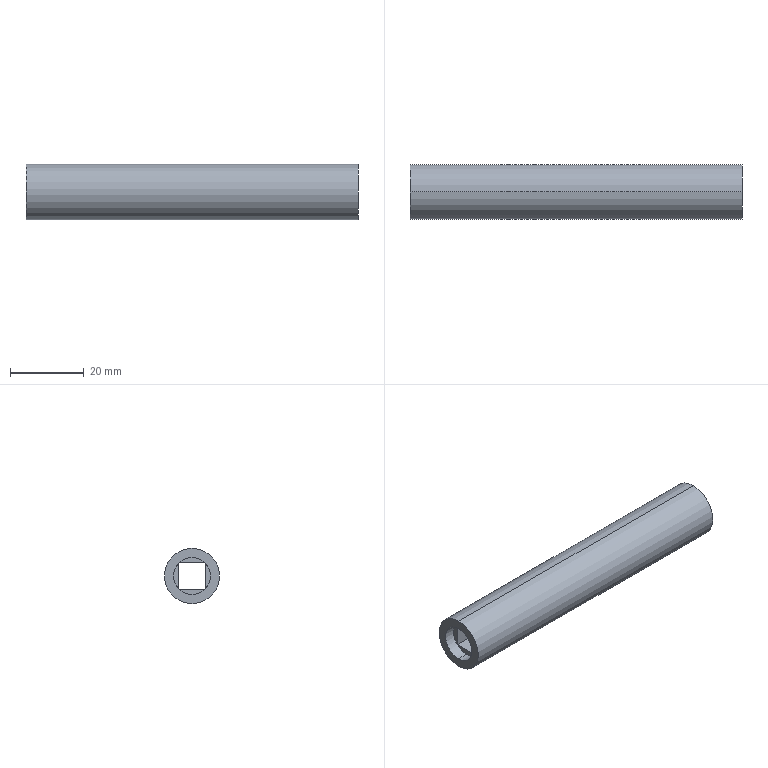Part | STEP file | Handle B | 1 solid | 18 faces | box 90 x 15 x 15 mm | volume 11283 mm3 | plane 14 | cylinder 4 | commonest cylinder face diameters 10 x2 15 x2
STEP:
#1=CARTESIAN_POINT('',(0.,0.,0.));
#2=DIRECTION('',(0.,0.,1.));
#3=DIRECTION('',(1.,0.,0.));
#4=AXIS2_PLACEMENT_3D('',#1,#2,#3);
#5=CARTESIAN_POINT('',(90.,0.,7.5));
#6=VERTEX_POINT('',#5);
#7=CARTESIAN_POINT('',(90.,0.,-7.5));
#8=VERTEX_POINT('',#7);
#9=CARTESIAN_POINT('',(90.,0.,0.));
#10=DIRECTION('',(-1.,0.,0.));
#11=DIRECTION('',(0.,0.,1.));
#12=AXIS2_PLACEMENT_3D('',#9,#10,#11);
#13=CIRCLE('',#12,7.5);
#14=CARTESIAN_POINT('',(0.,0.,0.));
#15=DIRECTION('',(-1.,0.,0.));
#16=DIRECTION('',(0.,0.,1.));
#17=AXIS2_PLACEMENT_3D('',#14,#15,#16);
#18=CYLINDRICAL_SURFACE('',#17,7.5);
#19=CARTESIAN_POINT('',(0.,-90.));
#20=DIRECTION('',(1.,0.));
#21=VECTOR('',#20,1.);
#22=LINE('',#19,#21);
#23=(GEOMETRIC_REPRESENTATION_CONTEXT(2)PARAMETRIC_REPRESENTATION_CONTEXT()REPRESENTATION_CONTEXT('',''));
#24=DEFINITIONAL_REPRESENTATION('',(#22),#23);
#25=PCURVE('',#18,#24);
#26=CARTESIAN_POINT('',(90.,7.5,0.));
#27=DIRECTION('',(-1.,0.,0.));
#28=DIRECTION('',(0.,0.,1.));
#29=AXIS2_PLACEMENT_3D('',#26,#27,#28);
#30=PLANE('',#29);
#31=CARTESIAN_POINT('',(0.,-7.5));
#32=DIRECTION('',(1.,0.));
#33=AXIS2_PLACEMENT_2D('',#31,#32);
#34=CIRCLE('',#33,7.5);
#35=(GEOMETRIC_REPRESENTATION_CONTEXT(2)PARAMETRIC_REPRESENTATION_CONTEXT()REPRESENTATION_CONTEXT('',''));
#36=DEFINITIONAL_REPRESENTATION('',(#34),#35);
#37=PCURVE('',#30,#36);
#38=SURFACE_CURVE('',#13,(#25,#37),.PCURVE_S1.);
#39=EDGE_CURVE('',#6,#8,#38,.T.);
#40=ORIENTED_EDGE('',*,*,#39,.T.);
#41=CARTESIAN_POINT('',(0.,0.,-7.5));
#42=VERTEX_POINT('',#41);
#43=CARTESIAN_POINT('',(0.,0.,-7.5));
#44=DIRECTION('',(-1.,0.,0.));
#45=VECTOR('',#44,1.);
#46=LINE('',#43,#45);
#47=CARTESIAN_POINT('',(3.142,0.));
#48=DIRECTION('',(0.,1.));
#49=VECTOR('',#48,1.);
#50=LINE('',#47,#49);
#51=(GEOMETRIC_REPRESENTATION_CONTEXT(2)PARAMETRIC_REPRESENTATION_CONTEXT()REPRESENTATION_CONTEXT('',''));
#52=DEFINITIONAL_REPRESENTATION('',(#50),#51);
#53=PCURVE('',#18,#52);
#54=CARTESIAN_POINT('',(0.,0.,0.));
#55=DIRECTION('',(-1.,0.,0.));
#56=DIRECTION('',(0.,0.,1.));
#57=AXIS2_PLACEMENT_3D('',#54,#55,#56);
#58=CYLINDRICAL_SURFACE('',#57,7.5);
#59=CARTESIAN_POINT('',(3.142,0.));
#60=DIRECTION('',(0.,1.));
#61=VECTOR('',#60,1.);
#62=LINE('',#59,#61);
#63=(GEOMETRIC_REPRESENTATION_CONTEXT(2)PARAMETRIC_REPRESENTATION_CONTEXT()REPRESENTATION_CONTEXT('',''));
#64=DEFINITIONAL_REPRESENTATION('',(#62),#63);
#65=PCURVE('',#58,#64);
#66=SURFACE_CURVE('',#46,(#53,#65),.PCURVE_S1.);
#67=EDGE_CURVE('',#8,#42,#66,.T.);
#68=ORIENTED_EDGE('',*,*,#67,.T.);
#69=CARTESIAN_POINT('',(0.,0.,7.5));
#70=VERTEX_POINT('',#69);
#71=CARTESIAN_POINT('',(0.,0.,0.));
#72=DIRECTION('',(-1.,0.,0.));
#73=DIRECTION('',(0.,0.,1.));
#74=AXIS2_PLACEMENT_3D('',#71,#72,#73);
#75=CIRCLE('',#74,7.5);
#76=CARTESIAN_POINT('',(0.,0.));
#77=DIRECTION('',(1.,0.));
#78=VECTOR('',#77,1.);
#79=LINE('',#76,#78);
#80=(GEOMETRIC_REPRESENTATION_CONTEXT(2)PARAMETRIC_REPRESENTATION_CONTEXT()REPRESENTATION_CONTEXT('',''));
#81=DEFINITIONAL_REPRESENTATION('',(#79),#80);
#82=PCURVE('',#18,#81);
#83=CARTESIAN_POINT('',(0.,5.,0.));
#84=DIRECTION('',(1.,0.,0.));
#85=DIRECTION('',(0.,0.,-1.));
#86=AXIS2_PLACEMENT_3D('',#83,#84,#85);
#87=PLANE('',#86);
#88=CARTESIAN_POINT('',(-7.5,-5.));
#89=CARTESIAN_POINT('',(-7.5,7.99));
#90=CARTESIAN_POINT('',(3.75,1.495));
#91=CARTESIAN_POINT('',(15.,-5.));
#92=CARTESIAN_POINT('',(3.75,-11.495));
#93=CARTESIAN_POINT('',(-7.5,-17.99));
#94=CARTESIAN_POINT('',(-7.5,-5.));
#95=(BOUNDED_CURVE()B_SPLINE_CURVE(2,(#88,#89,#90,#91,#92,#93,#94),.UNSPECIFIED.,.T.,.F.)B_SPLINE_CURVE_WITH_KNOTS((1,2,2,2,2,1),(-2.094,0.,2.094,4.189,6.283,8.378),.UNSPECIFIED.)CURVE()GEOMETRIC_REPRESENTATION_ITEM()RATIONAL_B_SPLINE_CURVE((1.,0.5,1.,0.5,1.,0.5,1.))REPRESENTATION_ITEM(''));
#96=(GEOMETRIC_REPRESENTATION_CONTEXT(2)PARAMETRIC_REPRESENTATION_CONTEXT()REPRESENTATION_CONTEXT('',''));
#97=DEFINITIONAL_REPRESENTATION('',(#95),#96);
#98=PCURVE('',#87,#97);
#99=SURFACE_CURVE('',#75,(#82,#98),.PCURVE_S1.);
#100=EDGE_CURVE('',#70,#42,#99,.T.);
#101=ORIENTED_EDGE('',*,*,#100,.F.);
#102=CARTESIAN_POINT('',(0.,0.,7.5));
#103=DIRECTION('',(-1.,0.,0.));
#104=VECTOR('',#103,1.);
#105=LINE('',#102,#104);
#106=CARTESIAN_POINT('',(0.,0.));
#107=DIRECTION('',(0.,1.));
#108=VECTOR('',#107,1.);
#109=LINE('',#106,#108);
#110=(GEOMETRIC_REPRESENTATION_CONTEXT(2)PARAMETRIC_REPRESENTATION_CONTEXT()REPRESENTATION_CONTEXT('',''));
#111=DEFINITIONAL_REPRESENTATION('',(#109),#110);
#112=PCURVE('',#18,#111);
#113=CARTESIAN_POINT('',(6.283,0.));
#114=DIRECTION('',(0.,1.));
#115=VECTOR('',#114,1.);
#116=LINE('',#113,#115);
#117=(GEOMETRIC_REPRESENTATION_CONTEXT(2)PARAMETRIC_REPRESENTATION_CONTEXT()REPRESENTATION_CONTEXT('',''));
#118=DEFINITIONAL_REPRESENTATION('',(#116),#117);
#119=PCURVE('',#58,#118);
#120=SURFACE_CURVE('',#105,(#112,#119),.PCURVE_S1.);
#121=EDGE_CURVE('',#6,#70,#120,.T.);
#122=ORIENTED_EDGE('',*,*,#121,.F.);
#123=EDGE_LOOP('',(#40,#68,#101,#122));
#124=FACE_BOUND('',#123,.T.);
#125=ADVANCED_FACE('',(#124),#18,.T.);
#126=CARTESIAN_POINT('',(3.,-3.521,-3.55));
#127=VERTEX_POINT('',#126);
#128=CARTESIAN_POINT('',(3.,-3.55,-3.521));
#129=VERTEX_POINT('',#128);
#130=CARTESIAN_POINT('',(3.,0.,0.));
#131=DIRECTION('',(-1.,0.,0.));
#132=DIRECTION('',(0.,0.,1.));
#133=AXIS2_PLACEMENT_3D('',#130,#131,#132);
#134=CIRCLE('',#133,5.);
#135=CARTESIAN_POINT('',(0.,0.,0.));
#136=DIRECTION('',(-1.,0.,0.));
#137=DIRECTION('',(0.,0.,1.));
#138=AXIS2_PLACEMENT_3D('',#135,#136,#137);
#139=CYLINDRICAL_SURFACE('',#138,5.);
#140=CARTESIAN_POINT('',(0.,-3.));
#141=DIRECTION('',(1.,0.));
#142=VECTOR('',#141,1.);
#143=LINE('',#140,#142);
#144=(GEOMETRIC_REPRESENTATION_CONTEXT(2)PARAMETRIC_REPRESENTATION_CONTEXT()REPRESENTATION_CONTEXT('',''));
#145=DEFINITIONAL_REPRESENTATION('',(#143),#144);
#146=PCURVE('',#139,#145);
#147=CARTESIAN_POINT('',(3.,0.,0.));
#148=DIRECTION('',(1.,0.,0.));
#149=DIRECTION('',(0.,0.,-1.));
#150=AXIS2_PLACEMENT_3D('',#147,#148,#149);
#151=PLANE('',#150);
#152=CARTESIAN_POINT('',(-5.,0.));
#153=CARTESIAN_POINT('',(-5.,8.66));
#154=CARTESIAN_POINT('',(2.5,4.33));
#155=CARTESIAN_POINT('',(10.,0.));
#156=CARTESIAN_POINT('',(2.5,-4.33));
#157=CARTESIAN_POINT('',(-5.,-8.66));
#158=CARTESIAN_POINT('',(-5.,0.));
#159=(BOUNDED_CURVE()B_SPLINE_CURVE(2,(#152,#153,#154,#155,#156,#157,#158),.UNSPECIFIED.,.T.,.F.)B_SPLINE_CURVE_WITH_KNOTS((1,2,2,2,2,1),(-2.094,0.,2.094,4.189,6.283,8.378),.UNSPECIFIED.)CURVE()GEOMETRIC_REPRESENTATION_ITEM()RATIONAL_B_SPLINE_CURVE((1.,0.5,1.,0.5,1.,0.5,1.))REPRESENTATION_ITEM(''));
#160=(GEOMETRIC_REPRESENTATION_CONTEXT(2)PARAMETRIC_REPRESENTATION_CONTEXT()REPRESENTATION_CONTEXT('',''));
#161=DEFINITIONAL_REPRESENTATION('',(#159),#160);
#162=PCURVE('',#151,#161);
#163=SURFACE_CURVE('',#134,(#146,#162),.PCURVE_S1.);
#164=EDGE_CURVE('',#127,#129,#163,.T.);
#165=ORIENTED_EDGE('',*,*,#164,.T.);
#166=CARTESIAN_POINT('',(3.,-3.55,3.521));
#167=VERTEX_POINT('',#166);
#168=CARTESIAN_POINT('',(3.,0.,0.));
#169=DIRECTION('',(-1.,0.,0.));
#170=DIRECTION('',(0.,0.,1.));
#171=AXIS2_PLACEMENT_3D('',#168,#169,#170);
#172=CIRCLE('',#171,5.);
#173=CARTESIAN_POINT('',(0.,-3.));
#174=DIRECTION('',(1.,0.));
#175=VECTOR('',#174,1.);
#176=LINE('',#173,#175);
#177=(GEOMETRIC_REPRESENTATION_CONTEXT(2)PARAMETRIC_REPRESENTATION_CONTEXT()REPRESENTATION_CONTEXT('',''));
#178=DEFINITIONAL_REPRESENTATION('',(#176),#177);
#179=PCURVE('',#139,#178);
#180=CARTESIAN_POINT('',(3.,3.209,0.));
#181=DIRECTION('',(1.,0.,0.));
#182=DIRECTION('',(0.,0.,-1.));
#183=AXIS2_PLACEMENT_3D('',#180,#181,#182);
#184=PLANE('',#183);
#185=CARTESIAN_POINT('',(-5.,-3.209));
#186=CARTESIAN_POINT('',(-5.,5.452));
#187=CARTESIAN_POINT('',(2.5,1.121));
#188=CARTESIAN_POINT('',(10.,-3.209));
#189=CARTESIAN_POINT('',(2.5,-7.539));
#190=CARTESIAN_POINT('',(-5.,-11.869));
#191=CARTESIAN_POINT('',(-5.,-3.209));
#192=(BOUNDED_CURVE()B_SPLINE_CURVE(2,(#185,#186,#187,#188,#189,#190,#191),.UNSPECIFIED.,.T.,.F.)B_SPLINE_CURVE_WITH_KNOTS((1,2,2,2,2,1),(-2.094,0.,2.094,4.189,6.283,8.378),.UNSPECIFIED.)CURVE()GEOMETRIC_REPRESENTATION_ITEM()RATIONAL_B_SPLINE_CURVE((1.,0.5,1.,0.5,1.,0.5,1.))REPRESENTATION_ITEM(''));
#193=(GEOMETRIC_REPRESENTATION_CONTEXT(2)PARAMETRIC_REPRESENTATION_CONTEXT()REPRESENTATION_CONTEXT('',''));
#194=DEFINITIONAL_REPRESENTATION('',(#192),#193);
#195=PCURVE('',#184,#194);
#196=SURFACE_CURVE('',#172,(#179,#195),.PCURVE_S1.);
#197=EDGE_CURVE('',#129,#167,#196,.T.);
#198=ORIENTED_EDGE('',*,*,#197,.T.);
#199=CARTESIAN_POINT('',(3.,-3.521,3.55));
#200=VERTEX_POINT('',#199);
#201=CARTESIAN_POINT('',(3.,0.,0.));
#202=DIRECTION('',(-1.,0.,0.));
#203=DIRECTION('',(0.,0.,1.));
#204=AXIS2_PLACEMENT_3D('',#201,#202,#203);
#205=CIRCLE('',#204,5.);
#206=CARTESIAN_POINT('',(0.,-3.));
#207=DIRECTION('',(1.,0.));
#208=VECTOR('',#207,1.);
#209=LINE('',#206,#208);
#210=(GEOMETRIC_REPRESENTATION_CONTEXT(2)PARAMETRIC_REPRESENTATION_CONTEXT()REPRESENTATION_CONTEXT('',''));
#211=DEFINITIONAL_REPRESENTATION('',(#209),#210);
#212=PCURVE('',#139,#211);
#213=CARTESIAN_POINT('',(3.,0.,0.));
#214=DIRECTION('',(1.,0.,0.));
#215=DIRECTION('',(0.,0.,-1.));
#216=AXIS2_PLACEMENT_3D('',#213,#214,#215);
#217=PLANE('',#216);
#218=CARTESIAN_POINT('',(-5.,0.));
#219=CARTESIAN_POINT('',(-5.,8.66));
#220=CARTESIAN_POINT('',(2.5,4.33));
#221=CARTESIAN_POINT('',(10.,0.));
#222=CARTESIAN_POINT('',(2.5,-4.33));
#223=CARTESIAN_POINT('',(-5.,-8.66));
#224=CARTESIAN_POINT('',(-5.,0.));
#225=(BOUNDED_CURVE()B_SPLINE_CURVE(2,(#218,#219,#220,#221,#222,#223,#224),.UNSPECIFIED.,.T.,.F.)B_SPLINE_CURVE_WITH_KNOTS((1,2,2,2,2,1),(-2.094,0.,2.094,4.189,6.283,8.378),.UNSPECIFIED.)CURVE()GEOMETRIC_REPRESENTATION_ITEM()RATIONAL_B_SPLINE_CURVE((1.,0.5,1.,0.5,1.,0.5,1.))REPRESENTATION_ITEM(''));
#226=(GEOMETRIC_REPRESENTATION_CONTEXT(2)PARAMETRIC_REPRESENTATION_CONTEXT()REPRESENTATION_CONTEXT('',''));
#227=DEFINITIONAL_REPRESENTATION('',(#225),#226);
#228=PCURVE('',#217,#227);
#229=SURFACE_CURVE('',#205,(#212,#228),.PCURVE_S1.);
#230=EDGE_CURVE('',#167,#200,#229,.T.);
#231=ORIENTED_EDGE('',*,*,#230,.T.);
#232=CARTESIAN_POINT('',(3.,0.,5.));
#233=VERTEX_POINT('',#232);
#234=CARTESIAN_POINT('',(3.,0.,0.));
#235=DIRECTION('',(-1.,0.,0.));
#236=DIRECTION('',(0.,0.,1.));
#237=AXIS2_PLACEMENT_3D('',#234,#235,#236);
#238=CIRCLE('',#237,5.);
#239=CARTESIAN_POINT('',(0.,-3.));
#240=DIRECTION('',(1.,0.));
#241=VECTOR('',#240,1.);
#242=LINE('',#239,#241);
#243=(GEOMETRIC_REPRESENTATION_CONTEXT(2)PARAMETRIC_REPRESENTATION_CONTEXT()REPRESENTATION_CONTEXT('',''));
#244=DEFINITIONAL_REPRESENTATION('',(#242),#243);
#245=PCURVE('',#139,#244);
#246=CARTESIAN_POINT('',(3.,3.209,0.));
#247=DIRECTION('',(1.,0.,0.));
#248=DIRECTION('',(0.,0.,-1.));
#249=AXIS2_PLACEMENT_3D('',#246,#247,#248);
#250=PLANE('',#249);
#251=CARTESIAN_POINT('',(-5.,-3.209));
#252=CARTESIAN_POINT('',(-5.,5.452));
#253=CARTESIAN_POINT('',(2.5,1.121));
#254=CARTESIAN_POINT('',(10.,-3.209));
#255=CARTESIAN_POINT('',(2.5,-7.539));
#256=CARTESIAN_POINT('',(-5.,-11.869));
#257=CARTESIAN_POINT('',(-5.,-3.209));
#258=(BOUNDED_CURVE()B_SPLINE_CURVE(2,(#251,#252,#253,#254,#255,#256,#257),.UNSPECIFIED.,.T.,.F.)B_SPLINE_CURVE_WITH_KNOTS((1,2,2,2,2,1),(-2.094,0.,2.094,4.189,6.283,8.378),.UNSPECIFIED.)CURVE()GEOMETRIC_REPRESENTATION_ITEM()RATIONAL_B_SPLINE_CURVE((1.,0.5,1.,0.5,1.,0.5,1.))REPRESENTATION_ITEM(''));
#259=(GEOMETRIC_REPRESENTATION_CONTEXT(2)PARAMETRIC_REPRESENTATION_CONTEXT()REPRESENTATION_CONTEXT('',''));
#260=DEFINITIONAL_REPRESENTATION('',(#258),#259);
#261=PCURVE('',#250,#260);
#262=SURFACE_CURVE('',#238,(#245,#261),.PCURVE_S1.);
#263=EDGE_CURVE('',#200,#233,#262,.T.);
#264=ORIENTED_EDGE('',*,*,#263,.T.);
#265=CARTESIAN_POINT('',(0.,0.,5.));
#266=VERTEX_POINT('',#265);
#267=CARTESIAN_POINT('',(0.,0.,5.));
#268=DIRECTION('',(-1.,0.,0.));
#269=VECTOR('',#268,1.);
#270=LINE('',#267,#269);
#271=CARTESIAN_POINT('',(6.283,0.));
#272=DIRECTION('',(0.,1.));
#273=VECTOR('',#272,1.);
#274=LINE('',#271,#273);
#275=(GEOMETRIC_REPRESENTATION_CONTEXT(2)PARAMETRIC_REPRESENTATION_CONTEXT()REPRESENTATION_CONTEXT('',''));
#276=DEFINITIONAL_REPRESENTATION('',(#274),#275);
#277=PCURVE('',#139,#276);
#278=CARTESIAN_POINT('',(0.,0.,0.));
#279=DIRECTION('',(-1.,0.,0.));
#280=DIRECTION('',(0.,0.,1.));
#281=AXIS2_PLACEMENT_3D('',#278,#279,#280);
#282=CYLINDRICAL_SURFACE('',#281,5.);
#283=CARTESIAN_POINT('',(0.,0.));
#284=DIRECTION('',(0.,1.));
#285=VECTOR('',#284,1.);
#286=LINE('',#283,#285);
#287=(GEOMETRIC_REPRESENTATION_CONTEXT(2)PARAMETRIC_REPRESENTATION_CONTEXT()REPRESENTATION_CONTEXT('',''));
#288=DEFINITIONAL_REPRESENTATION('',(#286),#287);
#289=PCURVE('',#282,#288);
#290=SURFACE_CURVE('',#270,(#277,#289),.PCURVE_S1.);
#291=EDGE_CURVE('',#233,#266,#290,.T.);
#292=ORIENTED_EDGE('',*,*,#291,.T.);
#293=CARTESIAN_POINT('',(0.,0.,-5.));
#294=VERTEX_POINT('',#293);
#295=CARTESIAN_POINT('',(0.,0.,0.));
#296=DIRECTION('',(-1.,0.,0.));
#297=DIRECTION('',(0.,0.,1.));
#298=AXIS2_PLACEMENT_3D('',#295,#296,#297);
#299=CIRCLE('',#298,5.);
#300=CARTESIAN_POINT('',(0.,0.));
#301=DIRECTION('',(1.,0.));
#302=VECTOR('',#301,1.);
#303=LINE('',#300,#302);
#304=(GEOMETRIC_REPRESENTATION_CONTEXT(2)PARAMETRIC_REPRESENTATION_CONTEXT()REPRESENTATION_CONTEXT('',''));
#305=DEFINITIONAL_REPRESENTATION('',(#303),#304);
#306=PCURVE('',#139,#305);
#307=CARTESIAN_POINT('',(-5.,-5.));
#308=CARTESIAN_POINT('',(-5.,3.66));
#309=CARTESIAN_POINT('',(2.5,-0.6699));
#310=CARTESIAN_POINT('',(10.,-5.));
#311=CARTESIAN_POINT('',(2.5,-9.33));
#312=CARTESIAN_POINT('',(-5.,-13.66));
#313=CARTESIAN_POINT('',(-5.,-5.));
#314=(BOUNDED_CURVE()B_SPLINE_CURVE(2,(#307,#308,#309,#310,#311,#312,#313),.UNSPECIFIED.,.T.,.F.)B_SPLINE_CURVE_WITH_KNOTS((1,2,2,2,2,1),(-2.094,0.,2.094,4.189,6.283,8.378),.UNSPECIFIED.)CURVE()GEOMETRIC_REPRESENTATION_ITEM()RATIONAL_B_SPLINE_CURVE((1.,0.5,1.,0.5,1.,0.5,1.))REPRESENTATION_ITEM(''));
#315=(GEOMETRIC_REPRESENTATION_CONTEXT(2)PARAMETRIC_REPRESENTATION_CONTEXT()REPRESENTATION_CONTEXT('',''));
#316=DEFINITIONAL_REPRESENTATION('',(#314),#315);
#317=PCURVE('',#87,#316);
#318=SURFACE_CURVE('',#299,(#306,#317),.PCURVE_S1.);
#319=EDGE_CURVE('',#294,#266,#318,.T.);
#320=ORIENTED_EDGE('',*,*,#319,.F.);
#321=CARTESIAN_POINT('',(3.,0.,-5.));
#322=VERTEX_POINT('',#321);
#323=CARTESIAN_POINT('',(0.,0.,-5.));
#324=DIRECTION('',(-1.,0.,0.));
#325=VECTOR('',#324,1.);
#326=LINE('',#323,#325);
#327=CARTESIAN_POINT('',(3.142,0.));
#328=DIRECTION('',(0.,1.));
#329=VECTOR('',#328,1.);
#330=LINE('',#327,#329);
#331=(GEOMETRIC_REPRESENTATION_CONTEXT(2)PARAMETRIC_REPRESENTATION_CONTEXT()REPRESENTATION_CONTEXT('',''));
#332=DEFINITIONAL_REPRESENTATION('',(#330),#331);
#333=PCURVE('',#139,#332);
#334=CARTESIAN_POINT('',(3.142,0.));
#335=DIRECTION('',(0.,1.));
#336=VECTOR('',#335,1.);
#337=LINE('',#334,#336);
#338=(GEOMETRIC_REPRESENTATION_CONTEXT(2)PARAMETRIC_REPRESENTATION_CONTEXT()REPRESENTATION_CONTEXT('',''));
#339=DEFINITIONAL_REPRESENTATION('',(#337),#338);
#340=PCURVE('',#282,#339);
#341=SURFACE_CURVE('',#326,(#333,#340),.PCURVE_S1.);
#342=EDGE_CURVE('',#322,#294,#341,.T.);
#343=ORIENTED_EDGE('',*,*,#342,.F.);
#344=CARTESIAN_POINT('',(3.,0.,0.));
#345=DIRECTION('',(-1.,0.,0.));
#346=DIRECTION('',(0.,0.,1.));
#347=AXIS2_PLACEMENT_3D('',#344,#345,#346);
#348=CIRCLE('',#347,5.);
#349=CARTESIAN_POINT('',(0.,-3.));
#350=DIRECTION('',(1.,0.));
#351=VECTOR('',#350,1.);
#352=LINE('',#349,#351);
#353=(GEOMETRIC_REPRESENTATION_CONTEXT(2)PARAMETRIC_REPRESENTATION_CONTEXT()REPRESENTATION_CONTEXT('',''));
#354=DEFINITIONAL_REPRESENTATION('',(#352),#353);
#355=PCURVE('',#139,#354);
#356=CARTESIAN_POINT('',(3.,3.209,0.));
#357=DIRECTION('',(1.,0.,0.));
#358=DIRECTION('',(0.,0.,-1.));
#359=AXIS2_PLACEMENT_3D('',#356,#357,#358);
#360=PLANE('',#359);
#361=CARTESIAN_POINT('',(-5.,-3.209));
#362=CARTESIAN_POINT('',(-5.,5.452));
#363=CARTESIAN_POINT('',(2.5,1.121));
#364=CARTESIAN_POINT('',(10.,-3.209));
#365=CARTESIAN_POINT('',(2.5,-7.539));
#366=CARTESIAN_POINT('',(-5.,-11.869));
#367=CARTESIAN_POINT('',(-5.,-3.209));
#368=(BOUNDED_CURVE()B_SPLINE_CURVE(2,(#361,#362,#363,#364,#365,#366,#367),.UNSPECIFIED.,.T.,.F.)B_SPLINE_CURVE_WITH_KNOTS((1,2,2,2,2,1),(-2.094,0.,2.094,4.189,6.283,8.378),.UNSPECIFIED.)CURVE()GEOMETRIC_REPRESENTATION_ITEM()RATIONAL_B_SPLINE_CURVE((1.,0.5,1.,0.5,1.,0.5,1.))REPRESENTATION_ITEM(''));
#369=(GEOMETRIC_REPRESENTATION_CONTEXT(2)PARAMETRIC_REPRESENTATION_CONTEXT()REPRESENTATION_CONTEXT('',''));
#370=DEFINITIONAL_REPRESENTATION('',(#368),#369);
#371=PCURVE('',#360,#370);
#372=SURFACE_CURVE('',#348,(#355,#371),.PCURVE_S1.);
#373=EDGE_CURVE('',#322,#127,#372,.T.);
#374=ORIENTED_EDGE('',*,*,#373,.T.);
#375=EDGE_LOOP('',(#165,#198,#231,#264,#292,#320,#343,#374));
#376=FACE_BOUND('',#375,.F.);
#377=ADVANCED_FACE('',(#376),#139,.F.);
#378=ORIENTED_EDGE('',*,*,#263,.T.);
#379=CARTESIAN_POINT('',(3.,3.521,3.55));
#380=VERTEX_POINT('',#379);
#381=CARTESIAN_POINT('',(3.,0.,0.));
#382=DIRECTION('',(-1.,0.,0.));
#383=DIRECTION('',(0.,0.,1.));
#384=AXIS2_PLACEMENT_3D('',#381,#382,#383);
#385=CIRCLE('',#384,5.);
#386=CARTESIAN_POINT('',(-5.,-3.209));
#387=CARTESIAN_POINT('',(-5.,5.452));
#388=CARTESIAN_POINT('',(2.5,1.121));
#389=CARTESIAN_POINT('',(10.,-3.209));
#390=CARTESIAN_POINT('',(2.5,-7.539));
#391=CARTESIAN_POINT('',(-5.,-11.869));
#392=CARTESIAN_POINT('',(-5.,-3.209));
#393=(BOUNDED_CURVE()B_SPLINE_CURVE(2,(#386,#387,#388,#389,#390,#391,#392),.UNSPECIFIED.,.T.,.F.)B_SPLINE_CURVE_WITH_KNOTS((1,2,2,2,2,1),(-2.094,0.,2.094,4.189,6.283,8.378),.UNSPECIFIED.)CURVE()GEOMETRIC_REPRESENTATION_ITEM()RATIONAL_B_SPLINE_CURVE((1.,0.5,1.,0.5,1.,0.5,1.))REPRESENTATION_ITEM(''));
#394=(GEOMETRIC_REPRESENTATION_CONTEXT(2)PARAMETRIC_REPRESENTATION_CONTEXT()REPRESENTATION_CONTEXT('',''));
#395=DEFINITIONAL_REPRESENTATION('',(#393),#394);
#396=PCURVE('',#250,#395);
#397=CARTESIAN_POINT('',(0.,-3.));
#398=DIRECTION('',(1.,0.));
#399=VECTOR('',#398,1.);
#400=LINE('',#397,#399);
#401=(GEOMETRIC_REPRESENTATION_CONTEXT(2)PARAMETRIC_REPRESENTATION_CONTEXT()REPRESENTATION_CONTEXT('',''));
#402=DEFINITIONAL_REPRESENTATION('',(#400),#401);
#403=PCURVE('',#282,#402);
#404=SURFACE_CURVE('',#385,(#396,#403),.PCURVE_S1.);
#405=EDGE_CURVE('',#233,#380,#404,.T.);
#406=ORIENTED_EDGE('',*,*,#405,.T.);
#407=CARTESIAN_POINT('',(3.,-3.55,3.55));
#408=DIRECTION('',(0.,1.,0.));
#409=VECTOR('',#408,1.);
#410=LINE('',#407,#409);
#411=CARTESIAN_POINT('',(-3.55,-6.759));
#412=DIRECTION('',(0.,1.));
#413=VECTOR('',#412,1.);
#414=LINE('',#411,#413);
#415=(GEOMETRIC_REPRESENTATION_CONTEXT(2)PARAMETRIC_REPRESENTATION_CONTEXT()REPRESENTATION_CONTEXT('',''));
#416=DEFINITIONAL_REPRESENTATION('',(#414),#415);
#417=PCURVE('',#250,#416);
#418=CARTESIAN_POINT('',(98.,-3.55,3.55));
#419=DIRECTION('',(0.,0.,1.));
#420=DIRECTION('',(1.,0.,0.));
#421=AXIS2_PLACEMENT_3D('',#418,#419,#420);
#422=PLANE('',#421);
#423=CARTESIAN_POINT('',(-95.,0.));
#424=DIRECTION('',(0.,1.));
#425=VECTOR('',#424,1.);
#426=LINE('',#423,#425);
#427=(GEOMETRIC_REPRESENTATION_CONTEXT(2)PARAMETRIC_REPRESENTATION_CONTEXT()REPRESENTATION_CONTEXT('',''));
#428=DEFINITIONAL_REPRESENTATION('',(#426),#427);
#429=PCURVE('',#422,#428);
#430=SURFACE_CURVE('',#410,(#417,#429),.PCURVE_S1.);
#431=EDGE_CURVE('',#200,#380,#430,.T.);
#432=ORIENTED_EDGE('',*,*,#431,.F.);
#433=EDGE_LOOP('',(#378,#406,#432));
#434=FACE_BOUND('',#433,.T.);
#435=ADVANCED_FACE('',(#434),#250,.F.);
#436=ORIENTED_EDGE('',*,*,#197,.T.);
#437=CARTESIAN_POINT('',(3.,-3.55,-3.55));
#438=DIRECTION('',(0.,0.,1.));
#439=VECTOR('',#438,1.);
#440=LINE('',#437,#439);
#441=CARTESIAN_POINT('',(3.55,-6.759));
#442=DIRECTION('',(-1.,0.));
#443=VECTOR('',#442,1.);
#444=LINE('',#441,#443);
#445=(GEOMETRIC_REPRESENTATION_CONTEXT(2)PARAMETRIC_REPRESENTATION_CONTEXT()REPRESENTATION_CONTEXT('',''));
#446=DEFINITIONAL_REPRESENTATION('',(#444),#445);
#447=PCURVE('',#184,#446);
#448=CARTESIAN_POINT('',(98.,-3.55,-3.55));
#449=DIRECTION('',(0.,-1.,0.));
#450=DIRECTION('',(0.,0.,-1.));
#451=AXIS2_PLACEMENT_3D('',#448,#449,#450);
#452=PLANE('',#451);
#453=CARTESIAN_POINT('',(0.,-95.));
#454=DIRECTION('',(-1.,0.));
#455=VECTOR('',#454,1.);
#456=LINE('',#453,#455);
#457=(GEOMETRIC_REPRESENTATION_CONTEXT(2)PARAMETRIC_REPRESENTATION_CONTEXT()REPRESENTATION_CONTEXT('',''));
#458=DEFINITIONAL_REPRESENTATION('',(#456),#457);
#459=PCURVE('',#452,#458);
#460=SURFACE_CURVE('',#440,(#447,#459),.PCURVE_S1.);
#461=EDGE_CURVE('',#129,#167,#460,.T.);
#462=ORIENTED_EDGE('',*,*,#461,.F.);
#463=EDGE_LOOP('',(#436,#462));
#464=FACE_BOUND('',#463,.T.);
#465=ADVANCED_FACE('',(#464),#184,.F.);
#466=CARTESIAN_POINT('',(3.,3.521,-3.55));
#467=VERTEX_POINT('',#466);
#468=CARTESIAN_POINT('',(3.,0.,0.));
#469=DIRECTION('',(-1.,0.,0.));
#470=DIRECTION('',(0.,0.,1.));
#471=AXIS2_PLACEMENT_3D('',#468,#469,#470);
#472=CIRCLE('',#471,5.);
#473=CARTESIAN_POINT('',(-5.,-3.209));
#474=CARTESIAN_POINT('',(-5.,5.452));
#475=CARTESIAN_POINT('',(2.5,1.121));
#476=CARTESIAN_POINT('',(10.,-3.209));
#477=CARTESIAN_POINT('',(2.5,-7.539));
#478=CARTESIAN_POINT('',(-5.,-11.869));
#479=CARTESIAN_POINT('',(-5.,-3.209));
#480=(BOUNDED_CURVE()B_SPLINE_CURVE(2,(#473,#474,#475,#476,#477,#478,#479),.UNSPECIFIED.,.T.,.F.)B_SPLINE_CURVE_WITH_KNOTS((1,2,2,2,2,1),(-2.094,0.,2.094,4.189,6.283,8.378),.UNSPECIFIED.)CURVE()GEOMETRIC_REPRESENTATION_ITEM()RATIONAL_B_SPLINE_CURVE((1.,0.5,1.,0.5,1.,0.5,1.))REPRESENTATION_ITEM(''));
#481=(GEOMETRIC_REPRESENTATION_CONTEXT(2)PARAMETRIC_REPRESENTATION_CONTEXT()REPRESENTATION_CONTEXT('',''));
#482=DEFINITIONAL_REPRESENTATION('',(#480),#481);
#483=PCURVE('',#360,#482);
#484=CARTESIAN_POINT('',(0.,-3.));
#485=DIRECTION('',(1.,0.));
#486=VECTOR('',#485,1.);
#487=LINE('',#484,#486);
#488=(GEOMETRIC_REPRESENTATION_CONTEXT(2)PARAMETRIC_REPRESENTATION_CONTEXT()REPRESENTATION_CONTEXT('',''));
#489=DEFINITIONAL_REPRESENTATION('',(#487),#488);
#490=PCURVE('',#282,#489);
#491=SURFACE_CURVE('',#472,(#483,#490),.PCURVE_S1.);
#492=EDGE_CURVE('',#467,#322,#491,.T.);
#493=ORIENTED_EDGE('',*,*,#492,.T.);
#494=ORIENTED_EDGE('',*,*,#373,.T.);
#495=CARTESIAN_POINT('',(3.,-3.55,-3.55));
#496=DIRECTION('',(0.,-1.,0.));
#497=VECTOR('',#496,1.);
#498=LINE('',#495,#497);
#499=CARTESIAN_POINT('',(3.55,-6.759));
#500=DIRECTION('',(0.,-1.));
#501=VECTOR('',#500,1.);
#502=LINE('',#499,#501);
#503=(GEOMETRIC_REPRESENTATION_CONTEXT(2)PARAMETRIC_REPRESENTATION_CONTEXT()REPRESENTATION_CONTEXT('',''));
#504=DEFINITIONAL_REPRESENTATION('',(#502),#503);
#505=PCURVE('',#360,#504);
#506=CARTESIAN_POINT('',(98.,-3.55,-3.55));
#507=DIRECTION('',(0.,0.,-1.));
#508=DIRECTION('',(-1.,0.,0.));
#509=AXIS2_PLACEMENT_3D('',#506,#507,#508);
#510=PLANE('',#509);
#511=CARTESIAN_POINT('',(95.,0.));
#512=DIRECTION('',(0.,-1.));
#513=VECTOR('',#512,1.);
#514=LINE('',#511,#513);
#515=(GEOMETRIC_REPRESENTATION_CONTEXT(2)PARAMETRIC_REPRESENTATION_CONTEXT()REPRESENTATION_CONTEXT('',''));
#516=DEFINITIONAL_REPRESENTATION('',(#514),#515);
#517=PCURVE('',#510,#516);
#518=SURFACE_CURVE('',#498,(#505,#517),.PCURVE_S1.);
#519=EDGE_CURVE('',#467,#127,#518,.T.);
#520=ORIENTED_EDGE('',*,*,#519,.F.);
#521=EDGE_LOOP('',(#493,#494,#520));
#522=FACE_BOUND('',#521,.T.);
#523=ADVANCED_FACE('',(#522),#360,.F.);
#524=CARTESIAN_POINT('',(90.,-3.55,-3.55));
#525=VERTEX_POINT('',#524);
#526=CARTESIAN_POINT('',(90.,-3.55,3.55));
#527=VERTEX_POINT('',#526);
#528=CARTESIAN_POINT('',(90.,-3.55,0.));
#529=DIRECTION('',(0.,0.,1.));
#530=VECTOR('',#529,1.);
#531=LINE('',#528,#530);
#532=CARTESIAN_POINT('',(0.,-11.05));
#533=DIRECTION('',(1.,0.));
#534=VECTOR('',#533,1.);
#535=LINE('',#532,#534);
#536=(GEOMETRIC_REPRESENTATION_CONTEXT(2)PARAMETRIC_REPRESENTATION_CONTEXT()REPRESENTATION_CONTEXT('',''));
#537=DEFINITIONAL_REPRESENTATION('',(#535),#536);
#538=PCURVE('',#30,#537);
#539=CARTESIAN_POINT('',(-3.55,-8.));
#540=DIRECTION('',(-1.,0.));
#541=VECTOR('',#540,1.);
#542=LINE('',#539,#541);
#543=(GEOMETRIC_REPRESENTATION_CONTEXT(2)PARAMETRIC_REPRESENTATION_CONTEXT()REPRESENTATION_CONTEXT('',''));
#544=DEFINITIONAL_REPRESENTATION('',(#542),#543);
#545=PCURVE('',#452,#544);
#546=SURFACE_CURVE('',#531,(#538,#545),.PCURVE_S1.);
#547=EDGE_CURVE('',#525,#527,#546,.T.);
#548=ORIENTED_EDGE('',*,*,#547,.T.);
#549=CARTESIAN_POINT('',(90.,3.55,3.55));
#550=VERTEX_POINT('',#549);
#551=CARTESIAN_POINT('',(90.,7.5,3.55));
#552=DIRECTION('',(0.,1.,0.));
#553=VECTOR('',#552,1.);
#554=LINE('',#551,#553);
#555=CARTESIAN_POINT('',(3.55,0.));
#556=DIRECTION('',(0.,1.));
#557=VECTOR('',#556,1.);
#558=LINE('',#555,#557);
#559=(GEOMETRIC_REPRESENTATION_CONTEXT(2)PARAMETRIC_REPRESENTATION_CONTEXT()REPRESENTATION_CONTEXT('',''));
#560=DEFINITIONAL_REPRESENTATION('',(#558),#559);
#561=PCURVE('',#30,#560);
#562=CARTESIAN_POINT('',(-8.,11.05));
#563=DIRECTION('',(0.,1.));
#564=VECTOR('',#563,1.);
#565=LINE('',#562,#564);
#566=(GEOMETRIC_REPRESENTATION_CONTEXT(2)PARAMETRIC_REPRESENTATION_CONTEXT()REPRESENTATION_CONTEXT('',''));
#567=DEFINITIONAL_REPRESENTATION('',(#565),#566);
#568=PCURVE('',#422,#567);
#569=SURFACE_CURVE('',#554,(#561,#568),.PCURVE_S1.);
#570=EDGE_CURVE('',#527,#550,#569,.T.);
#571=ORIENTED_EDGE('',*,*,#570,.T.);
#572=CARTESIAN_POINT('',(90.,3.55,-3.55));
#573=VERTEX_POINT('',#572);
#574=CARTESIAN_POINT('',(90.,3.55,0.));
#575=DIRECTION('',(0.,0.,-1.));
#576=VECTOR('',#575,1.);
#577=LINE('',#574,#576);
#578=CARTESIAN_POINT('',(0.,-3.95));
#579=DIRECTION('',(-1.,0.));
#580=VECTOR('',#579,1.);
#581=LINE('',#578,#580);
#582=(GEOMETRIC_REPRESENTATION_CONTEXT(2)PARAMETRIC_REPRESENTATION_CONTEXT()REPRESENTATION_CONTEXT('',''));
#583=DEFINITIONAL_REPRESENTATION('',(#581),#582);
#584=PCURVE('',#30,#583);
#585=CARTESIAN_POINT('',(98.,3.55,-3.55));
#586=DIRECTION('',(0.,1.,0.));
#587=DIRECTION('',(0.,0.,1.));
#588=AXIS2_PLACEMENT_3D('',#585,#586,#587);
#589=PLANE('',#588);
#590=CARTESIAN_POINT('',(3.55,-8.));
#591=DIRECTION('',(-1.,0.));
#592=VECTOR('',#591,1.);
#593=LINE('',#590,#592);
#594=(GEOMETRIC_REPRESENTATION_CONTEXT(2)PARAMETRIC_REPRESENTATION_CONTEXT()REPRESENTATION_CONTEXT('',''));
#595=DEFINITIONAL_REPRESENTATION('',(#593),#594);
#596=PCURVE('',#589,#595);
#597=SURFACE_CURVE('',#577,(#584,#596),.PCURVE_S1.);
#598=EDGE_CURVE('',#550,#573,#597,.T.);
#599=ORIENTED_EDGE('',*,*,#598,.T.);
#600=CARTESIAN_POINT('',(90.,7.5,-3.55));
#601=DIRECTION('',(0.,-1.,0.));
#602=VECTOR('',#601,1.);
#603=LINE('',#600,#602);
#604=CARTESIAN_POINT('',(-3.55,0.));
#605=DIRECTION('',(0.,-1.));
#606=VECTOR('',#605,1.);
#607=LINE('',#604,#606);
#608=(GEOMETRIC_REPRESENTATION_CONTEXT(2)PARAMETRIC_REPRESENTATION_CONTEXT()REPRESENTATION_CONTEXT('',''));
#609=DEFINITIONAL_REPRESENTATION('',(#607),#608);
#610=PCURVE('',#30,#609);
#611=CARTESIAN_POINT('',(8.,11.05));
#612=DIRECTION('',(0.,-1.));
#613=VECTOR('',#612,1.);
#614=LINE('',#611,#613);
#615=(GEOMETRIC_REPRESENTATION_CONTEXT(2)PARAMETRIC_REPRESENTATION_CONTEXT()REPRESENTATION_CONTEXT('',''));
#616=DEFINITIONAL_REPRESENTATION('',(#614),#615);
#617=PCURVE('',#510,#616);
#618=SURFACE_CURVE('',#603,(#610,#617),.PCURVE_S1.);
#619=EDGE_CURVE('',#573,#525,#618,.T.);
#620=ORIENTED_EDGE('',*,*,#619,.T.);
#621=EDGE_LOOP('',(#548,#571,#599,#620));
#622=FACE_BOUND('',#621,.T.);
#623=ORIENTED_EDGE('',*,*,#39,.F.);
#624=CARTESIAN_POINT('',(90.,0.,0.));
#625=DIRECTION('',(-1.,0.,0.));
#626=DIRECTION('',(0.,0.,1.));
#627=AXIS2_PLACEMENT_3D('',#624,#625,#626);
#628=CIRCLE('',#627,7.5);
#629=CARTESIAN_POINT('',(0.,-7.5));
#630=DIRECTION('',(1.,0.));
#631=AXIS2_PLACEMENT_2D('',#629,#630);
#632=CIRCLE('',#631,7.5);
#633=(GEOMETRIC_REPRESENTATION_CONTEXT(2)PARAMETRIC_REPRESENTATION_CONTEXT()REPRESENTATION_CONTEXT('',''));
#634=DEFINITIONAL_REPRESENTATION('',(#632),#633);
#635=PCURVE('',#30,#634);
#636=CARTESIAN_POINT('',(0.,-90.));
#637=DIRECTION('',(1.,0.));
#638=VECTOR('',#637,1.);
#639=LINE('',#636,#638);
#640=(GEOMETRIC_REPRESENTATION_CONTEXT(2)PARAMETRIC_REPRESENTATION_CONTEXT()REPRESENTATION_CONTEXT('',''));
#641=DEFINITIONAL_REPRESENTATION('',(#639),#640);
#642=PCURVE('',#58,#641);
#643=SURFACE_CURVE('',#628,(#635,#642),.PCURVE_S1.);
#644=EDGE_CURVE('',#8,#6,#643,.T.);
#645=ORIENTED_EDGE('',*,*,#644,.F.);
#646=EDGE_LOOP('',(#623,#645));
#647=FACE_BOUND('',#646,.T.);
#648=ADVANCED_FACE('',(#622,#647),#30,.F.);
#649=CARTESIAN_POINT('',(3.,3.55,3.521));
#650=VERTEX_POINT('',#649);
#651=CARTESIAN_POINT('',(3.,3.55,-3.521));
#652=VERTEX_POINT('',#651);
#653=CARTESIAN_POINT('',(3.,0.,0.));
#654=DIRECTION('',(-1.,0.,0.));
#655=DIRECTION('',(0.,0.,1.));
#656=AXIS2_PLACEMENT_3D('',#653,#654,#655);
#657=CIRCLE('',#656,5.);
#658=CARTESIAN_POINT('',(3.,3.209,0.));
#659=DIRECTION('',(1.,0.,0.));
#660=DIRECTION('',(0.,0.,-1.));
#661=AXIS2_PLACEMENT_3D('',#658,#659,#660);
#662=PLANE('',#661);
#663=CARTESIAN_POINT('',(-5.,-3.209));
#664=CARTESIAN_POINT('',(-5.,5.452));
#665=CARTESIAN_POINT('',(2.5,1.121));
#666=CARTESIAN_POINT('',(10.,-3.209));
#667=CARTESIAN_POINT('',(2.5,-7.539));
#668=CARTESIAN_POINT('',(-5.,-11.869));
#669=CARTESIAN_POINT('',(-5.,-3.209));
#670=(BOUNDED_CURVE()B_SPLINE_CURVE(2,(#663,#664,#665,#666,#667,#668,#669),.UNSPECIFIED.,.T.,.F.)B_SPLINE_CURVE_WITH_KNOTS((1,2,2,2,2,1),(-2.094,0.,2.094,4.189,6.283,8.378),.UNSPECIFIED.)CURVE()GEOMETRIC_REPRESENTATION_ITEM()RATIONAL_B_SPLINE_CURVE((1.,0.5,1.,0.5,1.,0.5,1.))REPRESENTATION_ITEM(''));
#671=(GEOMETRIC_REPRESENTATION_CONTEXT(2)PARAMETRIC_REPRESENTATION_CONTEXT()REPRESENTATION_CONTEXT('',''));
#672=DEFINITIONAL_REPRESENTATION('',(#670),#671);
#673=PCURVE('',#662,#672);
#674=CARTESIAN_POINT('',(0.,-3.));
#675=DIRECTION('',(1.,0.));
#676=VECTOR('',#675,1.);
#677=LINE('',#674,#676);
#678=(GEOMETRIC_REPRESENTATION_CONTEXT(2)PARAMETRIC_REPRESENTATION_CONTEXT()REPRESENTATION_CONTEXT('',''));
#679=DEFINITIONAL_REPRESENTATION('',(#677),#678);
#680=PCURVE('',#282,#679);
#681=SURFACE_CURVE('',#657,(#673,#680),.PCURVE_S1.);
#682=EDGE_CURVE('',#650,#652,#681,.T.);
#683=ORIENTED_EDGE('',*,*,#682,.T.);
#684=CARTESIAN_POINT('',(3.,3.55,-3.55));
#685=DIRECTION('',(0.,0.,-1.));
#686=VECTOR('',#685,1.);
#687=LINE('',#684,#686);
#688=CARTESIAN_POINT('',(3.55,0.3413));
#689=DIRECTION('',(1.,0.));
#690=VECTOR('',#689,1.);
#691=LINE('',#688,#690);
#692=(GEOMETRIC_REPRESENTATION_CONTEXT(2)PARAMETRIC_REPRESENTATION_CONTEXT()REPRESENTATION_CONTEXT('',''));
#693=DEFINITIONAL_REPRESENTATION('',(#691),#692);
#694=PCURVE('',#662,#693);
#695=CARTESIAN_POINT('',(0.,-95.));
#696=DIRECTION('',(-1.,0.));
#697=VECTOR('',#696,1.);
#698=LINE('',#695,#697);
#699=(GEOMETRIC_REPRESENTATION_CONTEXT(2)PARAMETRIC_REPRESENTATION_CONTEXT()REPRESENTATION_CONTEXT('',''));
#700=DEFINITIONAL_REPRESENTATION('',(#698),#699);
#701=PCURVE('',#589,#700);
#702=SURFACE_CURVE('',#687,(#694,#701),.PCURVE_S1.);
#703=EDGE_CURVE('',#650,#652,#702,.T.);
#704=ORIENTED_EDGE('',*,*,#703,.F.);
#705=EDGE_LOOP('',(#683,#704));
#706=FACE_BOUND('',#705,.T.);
#707=ADVANCED_FACE('',(#706),#662,.F.);
#708=CARTESIAN_POINT('',(0.,0.,0.));
#709=DIRECTION('',(-1.,0.,0.));
#710=DIRECTION('',(0.,0.,1.));
#711=AXIS2_PLACEMENT_3D('',#708,#709,#710);
#712=CIRCLE('',#711,5.);
#713=CARTESIAN_POINT('',(0.,0.));
#714=DIRECTION('',(1.,0.));
#715=VECTOR('',#714,1.);
#716=LINE('',#713,#715);
#717=(GEOMETRIC_REPRESENTATION_CONTEXT(2)PARAMETRIC_REPRESENTATION_CONTEXT()REPRESENTATION_CONTEXT('',''));
#718=DEFINITIONAL_REPRESENTATION('',(#716),#717);
#719=PCURVE('',#282,#718);
#720=CARTESIAN_POINT('',(-5.,-5.));
#721=CARTESIAN_POINT('',(-5.,3.66));
#722=CARTESIAN_POINT('',(2.5,-0.6699));
#723=CARTESIAN_POINT('',(10.,-5.));
#724=CARTESIAN_POINT('',(2.5,-9.33));
#725=CARTESIAN_POINT('',(-5.,-13.66));
#726=CARTESIAN_POINT('',(-5.,-5.));
#727=(BOUNDED_CURVE()B_SPLINE_CURVE(2,(#720,#721,#722,#723,#724,#725,#726),.UNSPECIFIED.,.T.,.F.)B_SPLINE_CURVE_WITH_KNOTS((1,2,2,2,2,1),(-2.094,0.,2.094,4.189,6.283,8.378),.UNSPECIFIED.)CURVE()GEOMETRIC_REPRESENTATION_ITEM()RATIONAL_B_SPLINE_CURVE((1.,0.5,1.,0.5,1.,0.5,1.))REPRESENTATION_ITEM(''));
#728=(GEOMETRIC_REPRESENTATION_CONTEXT(2)PARAMETRIC_REPRESENTATION_CONTEXT()REPRESENTATION_CONTEXT('',''));
#729=DEFINITIONAL_REPRESENTATION('',(#727),#728);
#730=PCURVE('',#87,#729);
#731=SURFACE_CURVE('',#712,(#719,#730),.PCURVE_S1.);
#732=EDGE_CURVE('',#266,#294,#731,.T.);
#733=ORIENTED_EDGE('',*,*,#732,.F.);
#734=ORIENTED_EDGE('',*,*,#291,.F.);
#735=ORIENTED_EDGE('',*,*,#405,.T.);
#736=CARTESIAN_POINT('',(3.,0.,0.));
#737=DIRECTION('',(-1.,0.,0.));
#738=DIRECTION('',(0.,0.,1.));
#739=AXIS2_PLACEMENT_3D('',#736,#737,#738);
#740=CIRCLE('',#739,5.);
#741=CARTESIAN_POINT('',(0.,-3.));
#742=DIRECTION('',(1.,0.));
#743=VECTOR('',#742,1.);
#744=LINE('',#741,#743);
#745=(GEOMETRIC_REPRESENTATION_CONTEXT(2)PARAMETRIC_REPRESENTATION_CONTEXT()REPRESENTATION_CONTEXT('',''));
#746=DEFINITIONAL_REPRESENTATION('',(#744),#745);
#747=PCURVE('',#282,#746);
#748=CARTESIAN_POINT('',(3.,0.,0.));
#749=DIRECTION('',(1.,0.,0.));
#750=DIRECTION('',(0.,0.,-1.));
#751=AXIS2_PLACEMENT_3D('',#748,#749,#750);
#752=PLANE('',#751);
#753=CARTESIAN_POINT('',(-5.,0.));
#754=CARTESIAN_POINT('',(-5.,8.66));
#755=CARTESIAN_POINT('',(2.5,4.33));
#756=CARTESIAN_POINT('',(10.,0.));
#757=CARTESIAN_POINT('',(2.5,-4.33));
#758=CARTESIAN_POINT('',(-5.,-8.66));
#759=CARTESIAN_POINT('',(-5.,0.));
#760=(BOUNDED_CURVE()B_SPLINE_CURVE(2,(#753,#754,#755,#756,#757,#758,#759),.UNSPECIFIED.,.T.,.F.)B_SPLINE_CURVE_WITH_KNOTS((1,2,2,2,2,1),(-2.094,0.,2.094,4.189,6.283,8.378),.UNSPECIFIED.)CURVE()GEOMETRIC_REPRESENTATION_ITEM()RATIONAL_B_SPLINE_CURVE((1.,0.5,1.,0.5,1.,0.5,1.))REPRESENTATION_ITEM(''));
#761=(GEOMETRIC_REPRESENTATION_CONTEXT(2)PARAMETRIC_REPRESENTATION_CONTEXT()REPRESENTATION_CONTEXT('',''));
#762=DEFINITIONAL_REPRESENTATION('',(#760),#761);
#763=PCURVE('',#752,#762);
#764=SURFACE_CURVE('',#740,(#747,#763),.PCURVE_S1.);
#765=EDGE_CURVE('',#380,#650,#764,.T.);
#766=ORIENTED_EDGE('',*,*,#765,.T.);
#767=ORIENTED_EDGE('',*,*,#682,.T.);
#768=CARTESIAN_POINT('',(3.,0.,0.));
#769=DIRECTION('',(-1.,0.,0.));
#770=DIRECTION('',(0.,0.,1.));
#771=AXIS2_PLACEMENT_3D('',#768,#769,#770);
#772=CIRCLE('',#771,5.);
#773=CARTESIAN_POINT('',(0.,-3.));
#774=DIRECTION('',(1.,0.));
#775=VECTOR('',#774,1.);
#776=LINE('',#773,#775);
#777=(GEOMETRIC_REPRESENTATION_CONTEXT(2)PARAMETRIC_REPRESENTATION_CONTEXT()REPRESENTATION_CONTEXT('',''));
#778=DEFINITIONAL_REPRESENTATION('',(#776),#777);
#779=PCURVE('',#282,#778);
#780=CARTESIAN_POINT('',(3.,0.,0.));
#781=DIRECTION('',(1.,0.,0.));
#782=DIRECTION('',(0.,0.,-1.));
#783=AXIS2_PLACEMENT_3D('',#780,#781,#782);
#784=PLANE('',#783);
#785=CARTESIAN_POINT('',(-5.,0.));
#786=CARTESIAN_POINT('',(-5.,8.66));
#787=CARTESIAN_POINT('',(2.5,4.33));
#788=CARTESIAN_POINT('',(10.,0.));
#789=CARTESIAN_POINT('',(2.5,-4.33));
#790=CARTESIAN_POINT('',(-5.,-8.66));
#791=CARTESIAN_POINT('',(-5.,0.));
#792=(BOUNDED_CURVE()B_SPLINE_CURVE(2,(#785,#786,#787,#788,#789,#790,#791),.UNSPECIFIED.,.T.,.F.)B_SPLINE_CURVE_WITH_KNOTS((1,2,2,2,2,1),(-2.094,0.,2.094,4.189,6.283,8.378),.UNSPECIFIED.)CURVE()GEOMETRIC_REPRESENTATION_ITEM()RATIONAL_B_SPLINE_CURVE((1.,0.5,1.,0.5,1.,0.5,1.))REPRESENTATION_ITEM(''));
#793=(GEOMETRIC_REPRESENTATION_CONTEXT(2)PARAMETRIC_REPRESENTATION_CONTEXT()REPRESENTATION_CONTEXT('',''));
#794=DEFINITIONAL_REPRESENTATION('',(#792),#793);
#795=PCURVE('',#784,#794);
#796=SURFACE_CURVE('',#772,(#779,#795),.PCURVE_S1.);
#797=EDGE_CURVE('',#652,#467,#796,.T.);
#798=ORIENTED_EDGE('',*,*,#797,.T.);
#799=ORIENTED_EDGE('',*,*,#492,.T.);
#800=ORIENTED_EDGE('',*,*,#342,.T.);
#801=EDGE_LOOP('',(#733,#734,#735,#766,#767,#798,#799,#800));
#802=FACE_BOUND('',#801,.F.);
#803=ADVANCED_FACE('',(#802),#282,.F.);
#804=ORIENTED_EDGE('',*,*,#732,.F.);
#805=ORIENTED_EDGE('',*,*,#319,.F.);
#806=EDGE_LOOP('',(#804,#805));
#807=FACE_BOUND('',#806,.T.);
#808=ORIENTED_EDGE('',*,*,#100,.T.);
#809=CARTESIAN_POINT('',(0.,0.,0.));
#810=DIRECTION('',(-1.,0.,0.));
#811=DIRECTION('',(0.,0.,1.));
#812=AXIS2_PLACEMENT_3D('',#809,#810,#811);
#813=CIRCLE('',#812,7.5);
#814=CARTESIAN_POINT('',(-7.5,-5.));
#815=CARTESIAN_POINT('',(-7.5,7.99));
#816=CARTESIAN_POINT('',(3.75,1.495));
#817=CARTESIAN_POINT('',(15.,-5.));
#818=CARTESIAN_POINT('',(3.75,-11.495));
#819=CARTESIAN_POINT('',(-7.5,-17.99));
#820=CARTESIAN_POINT('',(-7.5,-5.));
#821=(BOUNDED_CURVE()B_SPLINE_CURVE(2,(#814,#815,#816,#817,#818,#819,#820),.UNSPECIFIED.,.T.,.F.)B_SPLINE_CURVE_WITH_KNOTS((1,2,2,2,2,1),(-2.094,0.,2.094,4.189,6.283,8.378),.UNSPECIFIED.)CURVE()GEOMETRIC_REPRESENTATION_ITEM()RATIONAL_B_SPLINE_CURVE((1.,0.5,1.,0.5,1.,0.5,1.))REPRESENTATION_ITEM(''));
#822=(GEOMETRIC_REPRESENTATION_CONTEXT(2)PARAMETRIC_REPRESENTATION_CONTEXT()REPRESENTATION_CONTEXT('',''));
#823=DEFINITIONAL_REPRESENTATION('',(#821),#822);
#824=PCURVE('',#87,#823);
#825=CARTESIAN_POINT('',(0.,0.));
#826=DIRECTION('',(1.,0.));
#827=VECTOR('',#826,1.);
#828=LINE('',#825,#827);
#829=(GEOMETRIC_REPRESENTATION_CONTEXT(2)PARAMETRIC_REPRESENTATION_CONTEXT()REPRESENTATION_CONTEXT('',''));
#830=DEFINITIONAL_REPRESENTATION('',(#828),#829);
#831=PCURVE('',#58,#830);
#832=SURFACE_CURVE('',#813,(#824,#831),.PCURVE_S1.);
#833=EDGE_CURVE('',#42,#70,#832,.T.);
#834=ORIENTED_EDGE('',*,*,#833,.T.);
#835=EDGE_LOOP('',(#808,#834));
#836=FACE_BOUND('',#835,.T.);
#837=ADVANCED_FACE('',(#807,#836),#87,.F.);
#838=ORIENTED_EDGE('',*,*,#67,.F.);
#839=ORIENTED_EDGE('',*,*,#644,.T.);
#840=ORIENTED_EDGE('',*,*,#121,.T.);
#841=ORIENTED_EDGE('',*,*,#833,.F.);
#842=EDGE_LOOP('',(#838,#839,#840,#841));
#843=FACE_BOUND('',#842,.T.);
#844=ADVANCED_FACE('',(#843),#58,.T.);
#845=CARTESIAN_POINT('',(3.,-3.55,3.55));
#846=VERTEX_POINT('',#845);
#847=CARTESIAN_POINT('',(98.,-3.55,3.55));
#848=DIRECTION('',(-1.,0.,0.));
#849=VECTOR('',#848,1.);
#850=LINE('',#847,#849);
#851=CARTESIAN_POINT('',(0.,0.));
#852=DIRECTION('',(-1.,0.));
#853=VECTOR('',#852,1.);
#854=LINE('',#851,#853);
#855=(GEOMETRIC_REPRESENTATION_CONTEXT(2)PARAMETRIC_REPRESENTATION_CONTEXT()REPRESENTATION_CONTEXT('',''));
#856=DEFINITIONAL_REPRESENTATION('',(#854),#855);
#857=PCURVE('',#422,#856);
#858=CARTESIAN_POINT('',(-7.1,0.));
#859=DIRECTION('',(0.,-1.));
#860=VECTOR('',#859,1.);
#861=LINE('',#858,#860);
#862=(GEOMETRIC_REPRESENTATION_CONTEXT(2)PARAMETRIC_REPRESENTATION_CONTEXT()REPRESENTATION_CONTEXT('',''));
#863=DEFINITIONAL_REPRESENTATION('',(#861),#862);
#864=PCURVE('',#452,#863);
#865=SURFACE_CURVE('',#850,(#857,#864),.PCURVE_S1.);
#866=EDGE_CURVE('',#527,#846,#865,.T.);
#867=ORIENTED_EDGE('',*,*,#866,.T.);
#868=CARTESIAN_POINT('',(3.,-3.55,3.55));
#869=DIRECTION('',(0.,1.,0.));
#870=VECTOR('',#869,1.);
#871=LINE('',#868,#870);
#872=CARTESIAN_POINT('',(-95.,0.));
#873=DIRECTION('',(0.,1.));
#874=VECTOR('',#873,1.);
#875=LINE('',#872,#874);
#876=(GEOMETRIC_REPRESENTATION_CONTEXT(2)PARAMETRIC_REPRESENTATION_CONTEXT()REPRESENTATION_CONTEXT('',''));
#877=DEFINITIONAL_REPRESENTATION('',(#875),#876);
#878=PCURVE('',#422,#877);
#879=CARTESIAN_POINT('',(-3.55,-3.55));
#880=DIRECTION('',(0.,1.));
#881=VECTOR('',#880,1.);
#882=LINE('',#879,#881);
#883=(GEOMETRIC_REPRESENTATION_CONTEXT(2)PARAMETRIC_REPRESENTATION_CONTEXT()REPRESENTATION_CONTEXT('',''));
#884=DEFINITIONAL_REPRESENTATION('',(#882),#883);
#885=PCURVE('',#217,#884);
#886=SURFACE_CURVE('',#871,(#878,#885),.PCURVE_S1.);
#887=EDGE_CURVE('',#846,#200,#886,.T.);
#888=ORIENTED_EDGE('',*,*,#887,.T.);
#889=ORIENTED_EDGE('',*,*,#431,.T.);
#890=CARTESIAN_POINT('',(3.,3.55,3.55));
#891=VERTEX_POINT('',#890);
#892=CARTESIAN_POINT('',(3.,-3.55,3.55));
#893=DIRECTION('',(0.,1.,0.));
#894=VECTOR('',#893,1.);
#895=LINE('',#892,#894);
#896=CARTESIAN_POINT('',(-95.,0.));
#897=DIRECTION('',(0.,1.));
#898=VECTOR('',#897,1.);
#899=LINE('',#896,#898);
#900=(GEOMETRIC_REPRESENTATION_CONTEXT(2)PARAMETRIC_REPRESENTATION_CONTEXT()REPRESENTATION_CONTEXT('',''));
#901=DEFINITIONAL_REPRESENTATION('',(#899),#900);
#902=PCURVE('',#422,#901);
#903=CARTESIAN_POINT('',(-3.55,-3.55));
#904=DIRECTION('',(0.,1.));
#905=VECTOR('',#904,1.);
#906=LINE('',#903,#905);
#907=(GEOMETRIC_REPRESENTATION_CONTEXT(2)PARAMETRIC_REPRESENTATION_CONTEXT()REPRESENTATION_CONTEXT('',''));
#908=DEFINITIONAL_REPRESENTATION('',(#906),#907);
#909=PCURVE('',#752,#908);
#910=SURFACE_CURVE('',#895,(#902,#909),.PCURVE_S1.);
#911=EDGE_CURVE('',#380,#891,#910,.T.);
#912=ORIENTED_EDGE('',*,*,#911,.T.);
#913=CARTESIAN_POINT('',(98.,3.55,3.55));
#914=DIRECTION('',(-1.,0.,0.));
#915=VECTOR('',#914,1.);
#916=LINE('',#913,#915);
#917=CARTESIAN_POINT('',(0.,7.1));
#918=DIRECTION('',(-1.,0.));
#919=VECTOR('',#918,1.);
#920=LINE('',#917,#919);
#921=(GEOMETRIC_REPRESENTATION_CONTEXT(2)PARAMETRIC_REPRESENTATION_CONTEXT()REPRESENTATION_CONTEXT('',''));
#922=DEFINITIONAL_REPRESENTATION('',(#920),#921);
#923=PCURVE('',#422,#922);
#924=CARTESIAN_POINT('',(7.1,0.));
#925=DIRECTION('',(0.,-1.));
#926=VECTOR('',#925,1.);
#927=LINE('',#924,#926);
#928=(GEOMETRIC_REPRESENTATION_CONTEXT(2)PARAMETRIC_REPRESENTATION_CONTEXT()REPRESENTATION_CONTEXT('',''));
#929=DEFINITIONAL_REPRESENTATION('',(#927),#928);
#930=PCURVE('',#589,#929);
#931=SURFACE_CURVE('',#916,(#923,#930),.PCURVE_S1.);
#932=EDGE_CURVE('',#550,#891,#931,.T.);
#933=ORIENTED_EDGE('',*,*,#932,.F.);
#934=ORIENTED_EDGE('',*,*,#570,.F.);
#935=EDGE_LOOP('',(#867,#888,#889,#912,#933,#934));
#936=FACE_BOUND('',#935,.T.);
#937=ADVANCED_FACE('',(#936),#422,.F.);
#938=CARTESIAN_POINT('',(3.,-3.55,-3.55));
#939=VERTEX_POINT('',#938);
#940=CARTESIAN_POINT('',(98.,-3.55,-3.55));
#941=DIRECTION('',(-1.,0.,0.));
#942=VECTOR('',#941,1.);
#943=LINE('',#940,#942);
#944=CARTESIAN_POINT('',(0.,0.));
#945=DIRECTION('',(0.,-1.));
#946=VECTOR('',#945,1.);
#947=LINE('',#944,#946);
#948=(GEOMETRIC_REPRESENTATION_CONTEXT(2)PARAMETRIC_REPRESENTATION_CONTEXT()REPRESENTATION_CONTEXT('',''));
#949=DEFINITIONAL_REPRESENTATION('',(#947),#948);
#950=PCURVE('',#452,#949);
#951=CARTESIAN_POINT('',(0.,0.));
#952=DIRECTION('',(1.,0.));
#953=VECTOR('',#952,1.);
#954=LINE('',#951,#953);
#955=(GEOMETRIC_REPRESENTATION_CONTEXT(2)PARAMETRIC_REPRESENTATION_CONTEXT()REPRESENTATION_CONTEXT('',''));
#956=DEFINITIONAL_REPRESENTATION('',(#954),#955);
#957=PCURVE('',#510,#956);
#958=SURFACE_CURVE('',#943,(#950,#957),.PCURVE_S1.);
#959=EDGE_CURVE('',#525,#939,#958,.T.);
#960=ORIENTED_EDGE('',*,*,#959,.T.);
#961=CARTESIAN_POINT('',(3.,-3.55,-3.55));
#962=DIRECTION('',(0.,0.,1.));
#963=VECTOR('',#962,1.);
#964=LINE('',#961,#963);
#965=CARTESIAN_POINT('',(0.,-95.));
#966=DIRECTION('',(-1.,0.));
#967=VECTOR('',#966,1.);
#968=LINE('',#965,#967);
#969=(GEOMETRIC_REPRESENTATION_CONTEXT(2)PARAMETRIC_REPRESENTATION_CONTEXT()REPRESENTATION_CONTEXT('',''));
#970=DEFINITIONAL_REPRESENTATION('',(#968),#969);
#971=PCURVE('',#452,#970);
#972=CARTESIAN_POINT('',(3.55,-3.55));
#973=DIRECTION('',(-1.,0.));
#974=VECTOR('',#973,1.);
#975=LINE('',#972,#974);
#976=(GEOMETRIC_REPRESENTATION_CONTEXT(2)PARAMETRIC_REPRESENTATION_CONTEXT()REPRESENTATION_CONTEXT('',''));
#977=DEFINITIONAL_REPRESENTATION('',(#975),#976);
#978=PCURVE('',#151,#977);
#979=SURFACE_CURVE('',#964,(#971,#978),.PCURVE_S1.);
#980=EDGE_CURVE('',#939,#129,#979,.T.);
#981=ORIENTED_EDGE('',*,*,#980,.T.);
#982=ORIENTED_EDGE('',*,*,#461,.T.);
#983=CARTESIAN_POINT('',(3.,-3.55,-3.55));
#984=DIRECTION('',(0.,0.,1.));
#985=VECTOR('',#984,1.);
#986=LINE('',#983,#985);
#987=CARTESIAN_POINT('',(0.,-95.));
#988=DIRECTION('',(-1.,0.));
#989=VECTOR('',#988,1.);
#990=LINE('',#987,#989);
#991=(GEOMETRIC_REPRESENTATION_CONTEXT(2)PARAMETRIC_REPRESENTATION_CONTEXT()REPRESENTATION_CONTEXT('',''));
#992=DEFINITIONAL_REPRESENTATION('',(#990),#991);
#993=PCURVE('',#452,#992);
#994=CARTESIAN_POINT('',(3.55,-3.55));
#995=DIRECTION('',(-1.,0.));
#996=VECTOR('',#995,1.);
#997=LINE('',#994,#996);
#998=(GEOMETRIC_REPRESENTATION_CONTEXT(2)PARAMETRIC_REPRESENTATION_CONTEXT()REPRESENTATION_CONTEXT('',''));
#999=DEFINITIONAL_REPRESENTATION('',(#997),#998);
#1000=PCURVE('',#217,#999);
#1001=SURFACE_CURVE('',#986,(#993,#1000),.PCURVE_S1.);
#1002=EDGE_CURVE('',#167,#846,#1001,.T.);
#1003=ORIENTED_EDGE('',*,*,#1002,.T.);
#1004=ORIENTED_EDGE('',*,*,#866,.F.);
#1005=ORIENTED_EDGE('',*,*,#547,.F.);
#1006=EDGE_LOOP('',(#960,#981,#982,#1003,#1004,#1005));
#1007=FACE_BOUND('',#1006,.T.);
#1008=ADVANCED_FACE('',(#1007),#452,.F.);
#1009=CARTESIAN_POINT('',(3.,3.55,-3.55));
#1010=VERTEX_POINT('',#1009);
#1011=CARTESIAN_POINT('',(98.,3.55,-3.55));
#1012=DIRECTION('',(-1.,0.,0.));
#1013=VECTOR('',#1012,1.);
#1014=LINE('',#1011,#1013);
#1015=CARTESIAN_POINT('',(0.,7.1));
#1016=DIRECTION('',(1.,0.));
#1017=VECTOR('',#1016,1.);
#1018=LINE('',#1015,#1017);
#1019=(GEOMETRIC_REPRESENTATION_CONTEXT(2)PARAMETRIC_REPRESENTATION_CONTEXT()REPRESENTATION_CONTEXT('',''));
#1020=DEFINITIONAL_REPRESENTATION('',(#1018),#1019);
#1021=PCURVE('',#510,#1020);
#1022=CARTESIAN_POINT('',(0.,0.));
#1023=DIRECTION('',(0.,-1.));
#1024=VECTOR('',#1023,1.);
#1025=LINE('',#1022,#1024);
#1026=(GEOMETRIC_REPRESENTATION_CONTEXT(2)PARAMETRIC_REPRESENTATION_CONTEXT()REPRESENTATION_CONTEXT('',''));
#1027=DEFINITIONAL_REPRESENTATION('',(#1025),#1026);
#1028=PCURVE('',#589,#1027);
#1029=SURFACE_CURVE('',#1014,(#1021,#1028),.PCURVE_S1.);
#1030=EDGE_CURVE('',#573,#1010,#1029,.T.);
#1031=ORIENTED_EDGE('',*,*,#1030,.T.);
#1032=CARTESIAN_POINT('',(3.,-3.55,-3.55));
#1033=DIRECTION('',(0.,-1.,0.));
#1034=VECTOR('',#1033,1.);
#1035=LINE('',#1032,#1034);
#1036=CARTESIAN_POINT('',(95.,0.));
#1037=DIRECTION('',(0.,-1.));
#1038=VECTOR('',#1037,1.);
#1039=LINE('',#1036,#1038);
#1040=(GEOMETRIC_REPRESENTATION_CONTEXT(2)PARAMETRIC_REPRESENTATION_CONTEXT()REPRESENTATION_CONTEXT('',''));
#1041=DEFINITIONAL_REPRESENTATION('',(#1039),#1040);
#1042=PCURVE('',#510,#1041);
#1043=CARTESIAN_POINT('',(3.55,-3.55));
#1044=DIRECTION('',(0.,-1.));
#1045=VECTOR('',#1044,1.);
#1046=LINE('',#1043,#1045);
#1047=(GEOMETRIC_REPRESENTATION_CONTEXT(2)PARAMETRIC_REPRESENTATION_CONTEXT()REPRESENTATION_CONTEXT('',''));
#1048=DEFINITIONAL_REPRESENTATION('',(#1046),#1047);
#1049=PCURVE('',#784,#1048);
#1050=SURFACE_CURVE('',#1035,(#1042,#1049),.PCURVE_S1.);
#1051=EDGE_CURVE('',#1010,#467,#1050,.T.);
#1052=ORIENTED_EDGE('',*,*,#1051,.T.);
#1053=ORIENTED_EDGE('',*,*,#519,.T.);
#1054=CARTESIAN_POINT('',(3.,-3.55,-3.55));
#1055=DIRECTION('',(0.,-1.,0.));
#1056=VECTOR('',#1055,1.);
#1057=LINE('',#1054,#1056);
#1058=CARTESIAN_POINT('',(95.,0.));
#1059=DIRECTION('',(0.,-1.));
#1060=VECTOR('',#1059,1.);
#1061=LINE('',#1058,#1060);
#1062=(GEOMETRIC_REPRESENTATION_CONTEXT(2)PARAMETRIC_REPRESENTATION_CONTEXT()REPRESENTATION_CONTEXT('',''));
#1063=DEFINITIONAL_REPRESENTATION('',(#1061),#1062);
#1064=PCURVE('',#510,#1063);
#1065=CARTESIAN_POINT('',(3.55,-3.55));
#1066=DIRECTION('',(0.,-1.));
#1067=VECTOR('',#1066,1.);
#1068=LINE('',#1065,#1067);
#1069=(GEOMETRIC_REPRESENTATION_CONTEXT(2)PARAMETRIC_REPRESENTATION_CONTEXT()REPRESENTATION_CONTEXT('',''));
#1070=DEFINITIONAL_REPRESENTATION('',(#1068),#1069);
#1071=PCURVE('',#151,#1070);
#1072=SURFACE_CURVE('',#1057,(#1064,#1071),.PCURVE_S1.);
#1073=EDGE_CURVE('',#127,#939,#1072,.T.);
#1074=ORIENTED_EDGE('',*,*,#1073,.T.);
#1075=ORIENTED_EDGE('',*,*,#959,.F.);
#1076=ORIENTED_EDGE('',*,*,#619,.F.);
#1077=EDGE_LOOP('',(#1031,#1052,#1053,#1074,#1075,#1076));
#1078=FACE_BOUND('',#1077,.T.);
#1079=ADVANCED_FACE('',(#1078),#510,.F.);
#1080=ORIENTED_EDGE('',*,*,#932,.T.);
#1081=CARTESIAN_POINT('',(3.,3.55,-3.55));
#1082=DIRECTION('',(0.,0.,-1.));
#1083=VECTOR('',#1082,1.);
#1084=LINE('',#1081,#1083);
#1085=CARTESIAN_POINT('',(0.,-95.));
#1086=DIRECTION('',(-1.,0.));
#1087=VECTOR('',#1086,1.);
#1088=LINE('',#1085,#1087);
#1089=(GEOMETRIC_REPRESENTATION_CONTEXT(2)PARAMETRIC_REPRESENTATION_CONTEXT()REPRESENTATION_CONTEXT('',''));
#1090=DEFINITIONAL_REPRESENTATION('',(#1088),#1089);
#1091=PCURVE('',#589,#1090);
#1092=CARTESIAN_POINT('',(3.55,3.55));
#1093=DIRECTION('',(1.,0.));
#1094=VECTOR('',#1093,1.);
#1095=LINE('',#1092,#1094);
#1096=(GEOMETRIC_REPRESENTATION_CONTEXT(2)PARAMETRIC_REPRESENTATION_CONTEXT()REPRESENTATION_CONTEXT('',''));
#1097=DEFINITIONAL_REPRESENTATION('',(#1095),#1096);
#1098=PCURVE('',#752,#1097);
#1099=SURFACE_CURVE('',#1084,(#1091,#1098),.PCURVE_S1.);
#1100=EDGE_CURVE('',#891,#650,#1099,.T.);
#1101=ORIENTED_EDGE('',*,*,#1100,.T.);
#1102=ORIENTED_EDGE('',*,*,#703,.T.);
#1103=CARTESIAN_POINT('',(3.,3.55,-3.55));
#1104=DIRECTION('',(0.,0.,-1.));
#1105=VECTOR('',#1104,1.);
#1106=LINE('',#1103,#1105);
#1107=CARTESIAN_POINT('',(0.,-95.));
#1108=DIRECTION('',(-1.,0.));
#1109=VECTOR('',#1108,1.);
#1110=LINE('',#1107,#1109);
#1111=(GEOMETRIC_REPRESENTATION_CONTEXT(2)PARAMETRIC_REPRESENTATION_CONTEXT()REPRESENTATION_CONTEXT('',''));
#1112=DEFINITIONAL_REPRESENTATION('',(#1110),#1111);
#1113=PCURVE('',#589,#1112);
#1114=CARTESIAN_POINT('',(3.55,3.55));
#1115=DIRECTION('',(1.,0.));
#1116=VECTOR('',#1115,1.);
#1117=LINE('',#1114,#1116);
#1118=(GEOMETRIC_REPRESENTATION_CONTEXT(2)PARAMETRIC_REPRESENTATION_CONTEXT()REPRESENTATION_CONTEXT('',''));
#1119=DEFINITIONAL_REPRESENTATION('',(#1117),#1118);
#1120=PCURVE('',#784,#1119);
#1121=SURFACE_CURVE('',#1106,(#1113,#1120),.PCURVE_S1.);
#1122=EDGE_CURVE('',#652,#1010,#1121,.T.);
#1123=ORIENTED_EDGE('',*,*,#1122,.T.);
#1124=ORIENTED_EDGE('',*,*,#1030,.F.);
#1125=ORIENTED_EDGE('',*,*,#598,.F.);
#1126=EDGE_LOOP('',(#1080,#1101,#1102,#1123,#1124,#1125));
#1127=FACE_BOUND('',#1126,.T.);
#1128=ADVANCED_FACE('',(#1127),#589,.F.);
#1129=ORIENTED_EDGE('',*,*,#164,.T.);
#1130=ORIENTED_EDGE('',*,*,#980,.F.);
#1131=ORIENTED_EDGE('',*,*,#1073,.F.);
#1132=EDGE_LOOP('',(#1129,#1130,#1131));
#1133=FACE_BOUND('',#1132,.T.);
#1134=ADVANCED_FACE('',(#1133),#151,.T.);
#1135=ORIENTED_EDGE('',*,*,#230,.T.);
#1136=ORIENTED_EDGE('',*,*,#887,.F.);
#1137=ORIENTED_EDGE('',*,*,#1002,.F.);
#1138=EDGE_LOOP('',(#1135,#1136,#1137));
#1139=FACE_BOUND('',#1138,.T.);
#1140=ADVANCED_FACE('',(#1139),#217,.T.);
#1141=ORIENTED_EDGE('',*,*,#765,.T.);
#1142=ORIENTED_EDGE('',*,*,#1100,.F.);
#1143=ORIENTED_EDGE('',*,*,#911,.F.);
#1144=EDGE_LOOP('',(#1141,#1142,#1143));
#1145=FACE_BOUND('',#1144,.T.);
#1146=ADVANCED_FACE('',(#1145),#752,.T.);
#1147=ORIENTED_EDGE('',*,*,#797,.T.);
#1148=ORIENTED_EDGE('',*,*,#1051,.F.);
#1149=ORIENTED_EDGE('',*,*,#1122,.F.);
#1150=EDGE_LOOP('',(#1147,#1148,#1149));
#1151=FACE_BOUND('',#1150,.T.);
#1152=ADVANCED_FACE('',(#1151),#784,.T.);
#1153=CLOSED_SHELL('',(#125,#377,#435,#465,#523,#648,#707,#803,#837,#844,#937,#1008,#1079,#1128,#1134,#1140,#1146,#1152));
#1154=MANIFOLD_SOLID_BREP('',#1153);
#1155=(LENGTH_UNIT()NAMED_UNIT(*)SI_UNIT(.MILLI.,.METRE.));
#1156=UNCERTAINTY_MEASURE_WITH_UNIT(LENGTH_MEASURE(0.0000001),#1155,'','');
#1157=(NAMED_UNIT(*)PLANE_ANGLE_UNIT()SI_UNIT($,.RADIAN.));
#1158=(NAMED_UNIT(*)SI_UNIT($,.STERADIAN.)SOLID_ANGLE_UNIT());
#1159=(GEOMETRIC_REPRESENTATION_CONTEXT(3)GLOBAL_UNCERTAINTY_ASSIGNED_CONTEXT((#1156))GLOBAL_UNIT_ASSIGNED_CONTEXT((#1155,#1157,#1158))REPRESENTATION_CONTEXT('',''));
#1160=ADVANCED_BREP_SHAPE_REPRESENTATION('',(#4,#1154),#1159);